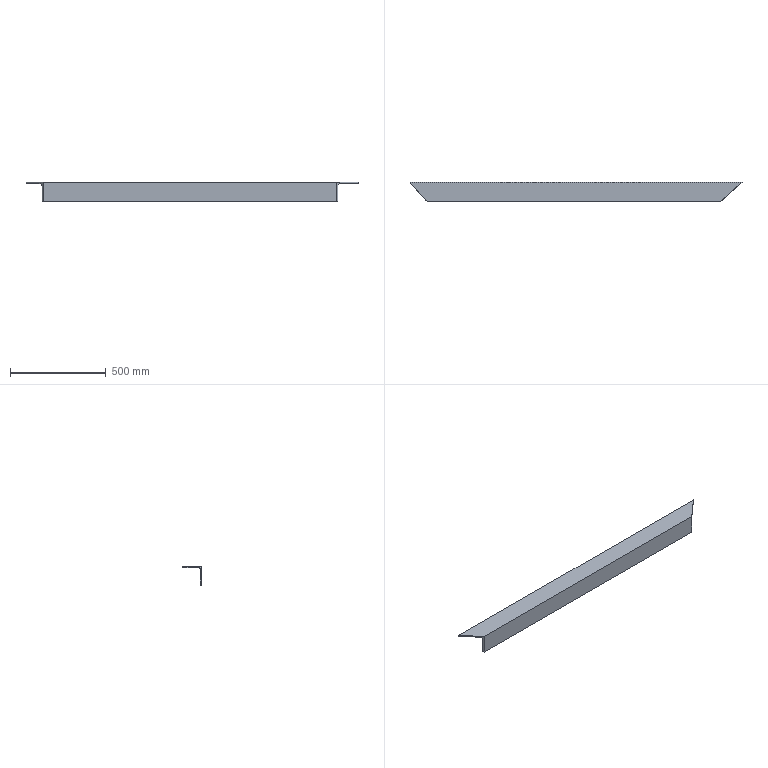Part | SolidWorks | features Extrusion 1, ICE 1 | 1 solid | 11 faces | box 1732 x 100 x 100 mm | volume 1888735 mm3 | plane 8 | cylinder 3 | commonest cylinder face diameters 5.4 x2 24 x1
STEP:
#1=CARTESIAN_POINT('',(-826.879,-32.,44.));
#2=VERTEX_POINT('',#1);
#3=CARTESIAN_POINT('',(-816.178,-44.,32.));
#4=VERTEX_POINT('',#3);
#5=CARTESIAN_POINT('',(-826.879,-32.,44.));
#6=CARTESIAN_POINT('',(-820.61,-39.029,44.));
#7=CARTESIAN_POINT('',(-816.178,-44.,39.029));
#8=CARTESIAN_POINT('',(-816.178,-44.,32.));
#9=(BOUNDED_CURVE()B_SPLINE_CURVE(3,(#5,#6,#7,#8),.UNSPECIFIED.,.F.,.T.)B_SPLINE_CURVE_WITH_KNOTS((4,4),(1.571,3.142),.UNSPECIFIED.)CURVE()GEOMETRIC_REPRESENTATION_ITEM()RATIONAL_B_SPLINE_CURVE((1.,0.8047,0.8047,1.))REPRESENTATION_ITEM(''));
#10=EDGE_CURVE('',#2,#4,#9,.T.);
#11=ORIENTED_EDGE('',*,*,#10,.F.);
#12=CARTESIAN_POINT('',(740.457,-32.,44.));
#13=VERTEX_POINT('',#12);
#14=CARTESIAN_POINT('',(900.,-32.,44.));
#15=DIRECTION('',(-1.,0.,0.));
#16=VECTOR('',#15,1000.);
#17=LINE('',#14,#16);
#18=EDGE_CURVE('',#13,#2,#17,.T.);
#19=ORIENTED_EDGE('',*,*,#18,.F.);
#20=CARTESIAN_POINT('',(727.,-44.,32.));
#21=VERTEX_POINT('',#20);
#22=CARTESIAN_POINT('',(727.,-44.,32.));
#23=CARTESIAN_POINT('',(727.,-44.,39.029));
#24=CARTESIAN_POINT('',(732.574,-39.029,44.));
#25=CARTESIAN_POINT('',(740.457,-32.,44.));
#26=(BOUNDED_CURVE()B_SPLINE_CURVE(3,(#22,#23,#24,#25),.UNSPECIFIED.,.F.,.F.)B_SPLINE_CURVE_WITH_KNOTS((4,4),(0.,1.571),.UNSPECIFIED.)CURVE()GEOMETRIC_REPRESENTATION_ITEM()RATIONAL_B_SPLINE_CURVE((1.,0.8047,0.8047,1.))REPRESENTATION_ITEM(''));
#27=EDGE_CURVE('',#21,#13,#26,.T.);
#28=ORIENTED_EDGE('',*,*,#27,.F.);
#29=CARTESIAN_POINT('',(900.,-44.,32.));
#30=DIRECTION('',(-1.,0.,0.));
#31=VECTOR('',#30,1000.);
#32=LINE('',#29,#31);
#33=EDGE_CURVE('',#21,#4,#32,.T.);
#34=ORIENTED_EDGE('',*,*,#33,.T.);
#35=EDGE_LOOP('',(#11,#19,#28,#34));
#36=FACE_OUTER_BOUND('',#35,.T.);
#37=CARTESIAN_POINT('',(900.,-32.,32.));
#38=DIRECTION('',(-1.,0.,0.));
#39=DIRECTION('',(0.,0.,1.));
#40=AXIS2_PLACEMENT_3D('',#37,#38,#39);
#41=CYLINDRICAL_SURFACE('',#40,12.);
#42=ADVANCED_FACE('',(#36),#41,.F.);
#43=CARTESIAN_POINT('',(-897.592,47.3,44.));
#44=VERTEX_POINT('',#43);
#45=CARTESIAN_POINT('',(-101.348,-845.626,44.));
#46=DIRECTION('',(0.6655,-0.7464,0.));
#47=VECTOR('',#46,1000.);
#48=LINE('',#45,#47);
#49=EDGE_CURVE('',#44,#2,#48,.T.);
#50=ORIENTED_EDGE('',*,*,#49,.F.);
#51=CARTESIAN_POINT('',(829.386,47.3,44.));
#52=VERTEX_POINT('',#51);
#53=CARTESIAN_POINT('',(900.,47.3,44.));
#54=DIRECTION('',(-1.,0.,0.));
#55=VECTOR('',#54,1000.);
#56=LINE('',#53,#55);
#57=EDGE_CURVE('',#52,#44,#56,.T.);
#58=ORIENTED_EDGE('',*,*,#57,.F.);
#59=CARTESIAN_POINT('',(868.722,82.376,44.));
#60=DIRECTION('',(0.7464,0.6655,0.));
#61=VECTOR('',#60,1000.);
#62=LINE('',#59,#61);
#63=EDGE_CURVE('',#13,#52,#62,.T.);
#64=ORIENTED_EDGE('',*,*,#63,.F.);
#65=ORIENTED_EDGE('',*,*,#18,.T.);
#66=EDGE_LOOP('',(#50,#58,#64,#65));
#67=FACE_OUTER_BOUND('',#66,.T.);
#68=CARTESIAN_POINT('',(900.,47.3,44.));
#69=DIRECTION('',(0.,0.,1.));
#70=DIRECTION('',(0.,-1.,0.));
#71=AXIS2_PLACEMENT_3D('',#68,#69,#70);
#72=PLANE('',#71);
#73=ADVANCED_FACE('',(#67),#72,.F.);
#74=CARTESIAN_POINT('',(-900.,50.,46.7));
#75=VERTEX_POINT('',#74);
#76=CARTESIAN_POINT('',(-900.,50.,46.7));
#77=CARTESIAN_POINT('',(-900.,50.,45.118));
#78=CARTESIAN_POINT('',(-899.003,48.882,44.));
#79=CARTESIAN_POINT('',(-897.592,47.3,44.));
#80=(BOUNDED_CURVE()B_SPLINE_CURVE(3,(#76,#77,#78,#79),.UNSPECIFIED.,.F.,.F.)B_SPLINE_CURVE_WITH_KNOTS((4,4),(0.,1.571),.UNSPECIFIED.)CURVE()GEOMETRIC_REPRESENTATION_ITEM()RATIONAL_B_SPLINE_CURVE((1.,0.8047,0.8047,1.))REPRESENTATION_ITEM(''));
#81=EDGE_CURVE('',#75,#44,#80,.T.);
#82=ORIENTED_EDGE('',*,*,#81,.F.);
#83=CARTESIAN_POINT('',(832.414,50.,46.7));
#84=VERTEX_POINT('',#83);
#85=CARTESIAN_POINT('',(900.,50.,46.7));
#86=DIRECTION('',(-1.,0.,0.));
#87=VECTOR('',#86,1000.);
#88=LINE('',#85,#87);
#89=EDGE_CURVE('',#84,#75,#88,.T.);
#90=ORIENTED_EDGE('',*,*,#89,.F.);
#91=CARTESIAN_POINT('',(829.386,47.3,44.));
#92=CARTESIAN_POINT('',(831.16,48.882,44.));
#93=CARTESIAN_POINT('',(832.414,50.,45.118));
#94=CARTESIAN_POINT('',(832.414,50.,46.7));
#95=(BOUNDED_CURVE()B_SPLINE_CURVE(3,(#91,#92,#93,#94),.UNSPECIFIED.,.F.,.F.)B_SPLINE_CURVE_WITH_KNOTS((4,4),(1.571,3.142),.UNSPECIFIED.)CURVE()GEOMETRIC_REPRESENTATION_ITEM()RATIONAL_B_SPLINE_CURVE((1.,0.8047,0.8047,1.))REPRESENTATION_ITEM(''));
#96=EDGE_CURVE('',#52,#84,#95,.T.);
#97=ORIENTED_EDGE('',*,*,#96,.F.);
#98=ORIENTED_EDGE('',*,*,#57,.T.);
#99=EDGE_LOOP('',(#82,#90,#97,#98));
#100=FACE_OUTER_BOUND('',#99,.T.);
#101=CARTESIAN_POINT('',(900.,47.3,46.7));
#102=DIRECTION('',(-1.,0.,0.));
#103=DIRECTION('',(0.,0.,1.));
#104=AXIS2_PLACEMENT_3D('',#101,#102,#103);
#105=CYLINDRICAL_SURFACE('',#104,2.7);
#106=ADVANCED_FACE('',(#100),#105,.T.);
#107=CARTESIAN_POINT('',(832.414,50.,50.));
#108=VERTEX_POINT('',#107);
#109=CARTESIAN_POINT('',(832.414,50.,-50.));
#110=DIRECTION('',(0.,0.,1.));
#111=VECTOR('',#110,1000.);
#112=LINE('',#109,#111);
#113=EDGE_CURVE('',#84,#108,#112,.T.);
#114=ORIENTED_EDGE('',*,*,#113,.F.);
#115=ORIENTED_EDGE('',*,*,#89,.T.);
#116=CARTESIAN_POINT('',(-900.,50.,50.));
#117=VERTEX_POINT('',#116);
#118=CARTESIAN_POINT('',(-900.,50.,50.));
#119=DIRECTION('',(0.,0.,1.));
#120=VECTOR('',#119,1000.);
#121=LINE('',#118,#120);
#122=EDGE_CURVE('',#75,#117,#121,.T.);
#123=ORIENTED_EDGE('',*,*,#122,.T.);
#124=CARTESIAN_POINT('',(900.,50.,50.));
#125=DIRECTION('',(-1.,0.,0.));
#126=VECTOR('',#125,1000.);
#127=LINE('',#124,#126);
#128=EDGE_CURVE('',#108,#117,#127,.T.);
#129=ORIENTED_EDGE('',*,*,#128,.F.);
#130=EDGE_LOOP('',(#114,#115,#123,#129));
#131=FACE_OUTER_BOUND('',#130,.T.);
#132=CARTESIAN_POINT('',(900.,50.,50.));
#133=DIRECTION('',(0.,-1.,0.));
#134=DIRECTION('',(0.,0.,-1.));
#135=AXIS2_PLACEMENT_3D('',#132,#133,#134);
#136=PLANE('',#135);
#137=ADVANCED_FACE('',(#131),#136,.F.);
#138=CARTESIAN_POINT('',(-810.828,-50.,50.));
#139=VERTEX_POINT('',#138);
#140=CARTESIAN_POINT('',(-900.,50.,50.));
#141=DIRECTION('',(0.6655,-0.7464,0.));
#142=VECTOR('',#141,1000.);
#143=LINE('',#140,#142);
#144=EDGE_CURVE('',#117,#139,#143,.T.);
#145=ORIENTED_EDGE('',*,*,#144,.T.);
#146=CARTESIAN_POINT('',(720.272,-50.,50.));
#147=VERTEX_POINT('',#146);
#148=CARTESIAN_POINT('',(900.,-50.,50.));
#149=DIRECTION('',(-1.,0.,0.));
#150=VECTOR('',#149,1000.);
#151=LINE('',#148,#150);
#152=EDGE_CURVE('',#147,#139,#151,.T.);
#153=ORIENTED_EDGE('',*,*,#152,.F.);
#154=CARTESIAN_POINT('',(-132.626,-810.55,50.));
#155=DIRECTION('',(0.7464,0.6655,0.));
#156=VECTOR('',#155,1000.);
#157=LINE('',#154,#156);
#158=EDGE_CURVE('',#147,#108,#157,.T.);
#159=ORIENTED_EDGE('',*,*,#158,.T.);
#160=ORIENTED_EDGE('',*,*,#128,.T.);
#161=EDGE_LOOP('',(#145,#153,#159,#160));
#162=FACE_OUTER_BOUND('',#161,.T.);
#163=CARTESIAN_POINT('',(900.,-50.,50.));
#164=DIRECTION('',(0.,0.,-1.));
#165=DIRECTION('',(0.,1.,0.));
#166=AXIS2_PLACEMENT_3D('',#163,#164,#165);
#167=PLANE('',#166);
#168=ADVANCED_FACE('',(#162),#167,.F.);
#169=CARTESIAN_POINT('',(-810.828,-50.,-50.));
#170=VERTEX_POINT('',#169);
#171=CARTESIAN_POINT('',(-810.828,-50.,-50.));
#172=DIRECTION('',(0.,0.,1.));
#173=VECTOR('',#172,1000.);
#174=LINE('',#171,#173);
#175=EDGE_CURVE('',#170,#139,#174,.T.);
#176=ORIENTED_EDGE('',*,*,#175,.F.);
#177=CARTESIAN_POINT('',(720.272,-50.,-50.));
#178=VERTEX_POINT('',#177);
#179=CARTESIAN_POINT('',(900.,-50.,-50.));
#180=DIRECTION('',(-1.,0.,0.));
#181=VECTOR('',#180,1000.);
#182=LINE('',#179,#181);
#183=EDGE_CURVE('',#178,#170,#182,.T.);
#184=ORIENTED_EDGE('',*,*,#183,.F.);
#185=CARTESIAN_POINT('',(720.272,-50.,-50.));
#186=DIRECTION('',(0.,0.,-1.));
#187=VECTOR('',#186,1000.);
#188=LINE('',#185,#187);
#189=EDGE_CURVE('',#147,#178,#188,.T.);
#190=ORIENTED_EDGE('',*,*,#189,.F.);
#191=ORIENTED_EDGE('',*,*,#152,.T.);
#192=EDGE_LOOP('',(#176,#184,#190,#191));
#193=FACE_OUTER_BOUND('',#192,.T.);
#194=CARTESIAN_POINT('',(900.,-50.,-50.));
#195=DIRECTION('',(0.,1.,0.));
#196=DIRECTION('',(0.,0.,1.));
#197=AXIS2_PLACEMENT_3D('',#194,#195,#196);
#198=PLANE('',#197);
#199=ADVANCED_FACE('',(#193),#198,.F.);
#200=CARTESIAN_POINT('',(-813.77,-46.7,-50.));
#201=VERTEX_POINT('',#200);
#202=CARTESIAN_POINT('',(-900.,50.,-50.));
#203=DIRECTION('',(0.6655,-0.7464,0.));
#204=VECTOR('',#203,1000.);
#205=LINE('',#202,#204);
#206=EDGE_CURVE('',#201,#170,#205,.T.);
#207=ORIENTED_EDGE('',*,*,#206,.F.);
#208=CARTESIAN_POINT('',(723.972,-46.7,-50.));
#209=VERTEX_POINT('',#208);
#210=CARTESIAN_POINT('',(900.,-46.7,-50.));
#211=DIRECTION('',(-1.,0.,0.));
#212=VECTOR('',#211,1000.);
#213=LINE('',#210,#212);
#214=EDGE_CURVE('',#209,#201,#213,.T.);
#215=ORIENTED_EDGE('',*,*,#214,.F.);
#216=CARTESIAN_POINT('',(-132.626,-810.55,-50.));
#217=DIRECTION('',(0.7464,0.6655,0.));
#218=VECTOR('',#217,1000.);
#219=LINE('',#216,#218);
#220=EDGE_CURVE('',#178,#209,#219,.T.);
#221=ORIENTED_EDGE('',*,*,#220,.F.);
#222=ORIENTED_EDGE('',*,*,#183,.T.);
#223=EDGE_LOOP('',(#207,#215,#221,#222));
#224=FACE_OUTER_BOUND('',#223,.T.);
#225=CARTESIAN_POINT('',(900.,-46.7,-50.));
#226=DIRECTION('',(0.,0.,1.));
#227=DIRECTION('',(1.,0.,0.));
#228=AXIS2_PLACEMENT_3D('',#225,#226,#227);
#229=PLANE('',#228);
#230=ADVANCED_FACE('',(#224),#229,.F.);
#231=CARTESIAN_POINT('',(-816.178,-44.,-47.3));
#232=VERTEX_POINT('',#231);
#233=CARTESIAN_POINT('',(-816.178,-44.,-47.3));
#234=CARTESIAN_POINT('',(-816.178,-44.,-48.882));
#235=CARTESIAN_POINT('',(-815.181,-45.118,-50.));
#236=CARTESIAN_POINT('',(-813.77,-46.7,-50.));
#237=(BOUNDED_CURVE()B_SPLINE_CURVE(3,(#233,#234,#235,#236),.UNSPECIFIED.,.F.,.F.)B_SPLINE_CURVE_WITH_KNOTS((4,4),(0.,1.571),.UNSPECIFIED.)CURVE()GEOMETRIC_REPRESENTATION_ITEM()RATIONAL_B_SPLINE_CURVE((1.,0.8047,0.8047,1.))REPRESENTATION_ITEM(''));
#238=EDGE_CURVE('',#232,#201,#237,.T.);
#239=ORIENTED_EDGE('',*,*,#238,.F.);
#240=CARTESIAN_POINT('',(727.,-44.,-47.3));
#241=VERTEX_POINT('',#240);
#242=CARTESIAN_POINT('',(900.,-44.,-47.3));
#243=DIRECTION('',(-1.,0.,0.));
#244=VECTOR('',#243,1000.);
#245=LINE('',#242,#244);
#246=EDGE_CURVE('',#241,#232,#245,.T.);
#247=ORIENTED_EDGE('',*,*,#246,.F.);
#248=CARTESIAN_POINT('',(723.972,-46.7,-50.));
#249=CARTESIAN_POINT('',(725.746,-45.118,-50.));
#250=CARTESIAN_POINT('',(727.,-44.,-48.882));
#251=CARTESIAN_POINT('',(727.,-44.,-47.3));
#252=(BOUNDED_CURVE()B_SPLINE_CURVE(3,(#248,#249,#250,#251),.UNSPECIFIED.,.F.,.F.)B_SPLINE_CURVE_WITH_KNOTS((4,4),(1.571,3.142),.UNSPECIFIED.)CURVE()GEOMETRIC_REPRESENTATION_ITEM()RATIONAL_B_SPLINE_CURVE((1.,0.8047,0.8047,1.))REPRESENTATION_ITEM(''));
#253=EDGE_CURVE('',#209,#241,#252,.T.);
#254=ORIENTED_EDGE('',*,*,#253,.F.);
#255=ORIENTED_EDGE('',*,*,#214,.T.);
#256=EDGE_LOOP('',(#239,#247,#254,#255));
#257=FACE_OUTER_BOUND('',#256,.T.);
#258=CARTESIAN_POINT('',(900.,-46.7,-47.3));
#259=DIRECTION('',(-1.,0.,0.));
#260=DIRECTION('',(0.,0.,1.));
#261=AXIS2_PLACEMENT_3D('',#258,#259,#260);
#262=CYLINDRICAL_SURFACE('',#261,2.7);
#263=ADVANCED_FACE('',(#257),#262,.T.);
#264=CARTESIAN_POINT('',(-816.178,-44.,32.));
#265=DIRECTION('',(0.,0.,-1.));
#266=VECTOR('',#265,1000.);
#267=LINE('',#264,#266);
#268=EDGE_CURVE('',#4,#232,#267,.T.);
#269=ORIENTED_EDGE('',*,*,#268,.F.);
#270=ORIENTED_EDGE('',*,*,#33,.F.);
#271=CARTESIAN_POINT('',(727.,-44.,32.));
#272=DIRECTION('',(0.,0.,1.));
#273=VECTOR('',#272,1000.);
#274=LINE('',#271,#273);
#275=EDGE_CURVE('',#241,#21,#274,.T.);
#276=ORIENTED_EDGE('',*,*,#275,.F.);
#277=ORIENTED_EDGE('',*,*,#246,.T.);
#278=EDGE_LOOP('',(#269,#270,#276,#277));
#279=FACE_OUTER_BOUND('',#278,.T.);
#280=CARTESIAN_POINT('',(900.,-44.,32.));
#281=DIRECTION('',(0.,-1.,0.));
#282=DIRECTION('',(0.,0.,-1.));
#283=AXIS2_PLACEMENT_3D('',#280,#281,#282);
#284=PLANE('',#283);
#285=ADVANCED_FACE('',(#279),#284,.F.);
#286=ORIENTED_EDGE('',*,*,#175,.T.);
#287=ORIENTED_EDGE('',*,*,#144,.F.);
#288=ORIENTED_EDGE('',*,*,#122,.F.);
#289=ORIENTED_EDGE('',*,*,#81,.T.);
#290=ORIENTED_EDGE('',*,*,#49,.T.);
#291=ORIENTED_EDGE('',*,*,#10,.T.);
#292=ORIENTED_EDGE('',*,*,#268,.T.);
#293=ORIENTED_EDGE('',*,*,#238,.T.);
#294=ORIENTED_EDGE('',*,*,#206,.T.);
#295=EDGE_LOOP('',(#286,#287,#288,#289,#290,#291,#292,#293,#294));
#296=FACE_OUTER_BOUND('',#295,.T.);
#297=CARTESIAN_POINT('',(-900.,50.,-50.));
#298=DIRECTION('',(-0.7464,-0.6655,0.));
#299=DIRECTION('',(0.6655,-0.7464,0.));
#300=AXIS2_PLACEMENT_3D('',#297,#298,#299);
#301=PLANE('',#300);
#302=ADVANCED_FACE('',(#296),#301,.T.);
#303=ORIENTED_EDGE('',*,*,#189,.T.);
#304=ORIENTED_EDGE('',*,*,#220,.T.);
#305=ORIENTED_EDGE('',*,*,#253,.T.);
#306=ORIENTED_EDGE('',*,*,#275,.T.);
#307=ORIENTED_EDGE('',*,*,#27,.T.);
#308=ORIENTED_EDGE('',*,*,#63,.T.);
#309=ORIENTED_EDGE('',*,*,#96,.T.);
#310=ORIENTED_EDGE('',*,*,#113,.T.);
#311=ORIENTED_EDGE('',*,*,#158,.F.);
#312=EDGE_LOOP('',(#303,#304,#305,#306,#307,#308,#309,#310,#311));
#313=FACE_OUTER_BOUND('',#312,.T.);
#314=CARTESIAN_POINT('',(-132.626,-810.55,-50.));
#315=DIRECTION('',(0.6655,-0.7464,0.));
#316=DIRECTION('',(0.7464,0.6655,0.));
#317=AXIS2_PLACEMENT_3D('',#314,#315,#316);
#318=PLANE('',#317);
#319=ADVANCED_FACE('',(#313),#318,.T.);
#320=CLOSED_SHELL('',(#42,#73,#106,#137,#168,#199,#230,#263,#285,#302,#319));
#321=MANIFOLD_SOLID_BREP('',#320);
#322=CARTESIAN_POINT('',(0.,0.,0.));
#323=DIRECTION('',(0.,0.,1.));
#324=DIRECTION('',(1.,0.,0.));
#325=AXIS2_PLACEMENT_3D('',#322,#323,#324);
#326=(LENGTH_UNIT()NAMED_UNIT(*)SI_UNIT(.MILLI.,.METRE.));
#327=UNCERTAINTY_MEASURE_WITH_UNIT(LENGTH_MEASURE(0.00001),#326,'','');
#328=(NAMED_UNIT(*)PLANE_ANGLE_UNIT()SI_UNIT($,.RADIAN.));
#329=(NAMED_UNIT(*)SI_UNIT($,.STERADIAN.)SOLID_ANGLE_UNIT());
#330=(GEOMETRIC_REPRESENTATION_CONTEXT(3)GLOBAL_UNCERTAINTY_ASSIGNED_CONTEXT((#327))GLOBAL_UNIT_ASSIGNED_CONTEXT((#326,#328,#329))REPRESENTATION_CONTEXT('',''));
#331=ADVANCED_BREP_SHAPE_REPRESENTATION('',(#321,#325),#330);